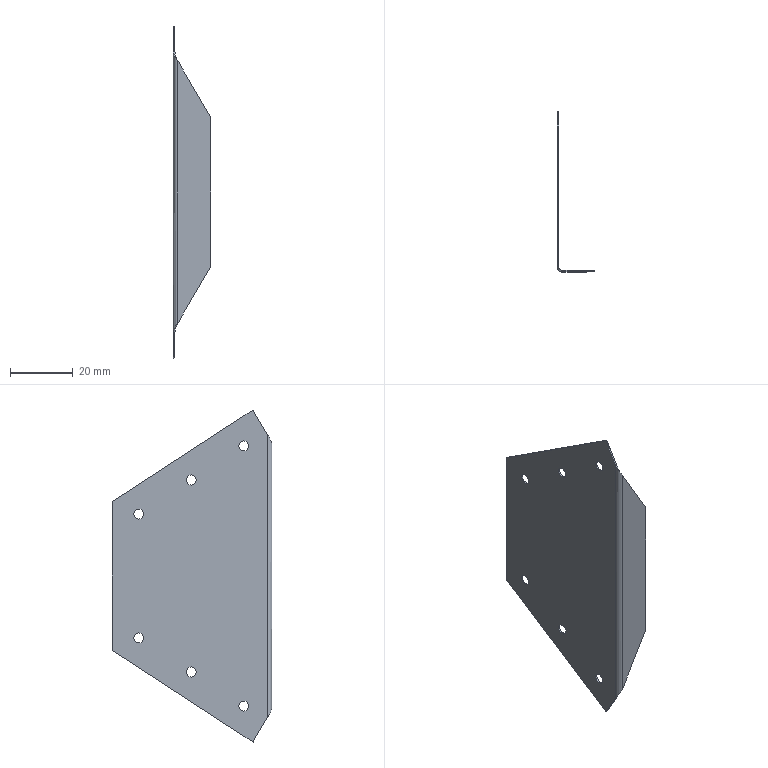Part | SolidWorks | features BaseBody 1 | 1 solid | 28 faces | box 12.018 x 51.018 x 106 mm | volume 2356 mm3 | cylinder 14 | plane 12 | spline 2 | commonest cylinder face diameters 3.2 x12 2 x1 3 x1
STEP:
#1=CARTESIAN_POINT('',(0.,-11.047,43.144));
#2=VERTEX_POINT('',#1);
#3=CARTESIAN_POINT('',(0.,-11.047,39.944));
#4=VERTEX_POINT('',#3);
#5=CARTESIAN_POINT('',(0.,-11.047,41.544));
#6=DIRECTION('',(1.,0.,0.));
#7=DIRECTION('',(0.,0.,1.));
#8=AXIS2_PLACEMENT_3D('',#5,#6,#7);
#9=CIRCLE('',#8,1.6);
#10=EDGE_CURVE('',#2,#4,#9,.T.);
#11=ORIENTED_EDGE('',*,*,#10,.T.);
#12=CARTESIAN_POINT('',(-0.5,-11.047,39.944));
#13=VERTEX_POINT('',#12);
#14=CARTESIAN_POINT('',(0.,-11.047,39.944));
#15=DIRECTION('',(-1.,0.,0.));
#16=VECTOR('',#15,1000.);
#17=LINE('',#14,#16);
#18=EDGE_CURVE('',#4,#13,#17,.T.);
#19=ORIENTED_EDGE('',*,*,#18,.T.);
#20=CARTESIAN_POINT('',(-0.5,-11.047,43.144));
#21=VERTEX_POINT('',#20);
#22=CARTESIAN_POINT('',(-0.5,-11.047,41.544));
#23=DIRECTION('',(-1.,0.,0.));
#24=DIRECTION('',(0.,0.,1.));
#25=AXIS2_PLACEMENT_3D('',#22,#23,#24);
#26=CIRCLE('',#25,1.6);
#27=EDGE_CURVE('',#13,#21,#26,.T.);
#28=ORIENTED_EDGE('',*,*,#27,.T.);
#29=CARTESIAN_POINT('',(0.,-11.047,43.144));
#30=DIRECTION('',(-1.,0.,0.));
#31=VECTOR('',#30,1000.);
#32=LINE('',#29,#31);
#33=EDGE_CURVE('',#2,#21,#32,.T.);
#34=ORIENTED_EDGE('',*,*,#33,.F.);
#35=EDGE_LOOP('',(#11,#19,#28,#34));
#36=FACE_OUTER_BOUND('',#35,.T.);
#37=CARTESIAN_POINT('',(0.,-11.047,41.544));
#38=DIRECTION('',(-1.,0.,0.));
#39=DIRECTION('',(0.,0.,1.));
#40=AXIS2_PLACEMENT_3D('',#37,#38,#39);
#41=CYLINDRICAL_SURFACE('',#40,1.6);
#42=ADVANCED_FACE('',(#36),#41,.F.);
#43=CARTESIAN_POINT('',(0.,-11.047,-43.144));
#44=VERTEX_POINT('',#43);
#45=CARTESIAN_POINT('',(0.,-11.047,-39.944));
#46=VERTEX_POINT('',#45);
#47=CARTESIAN_POINT('',(0.,-11.047,-41.544));
#48=DIRECTION('',(-1.,0.,0.));
#49=DIRECTION('',(0.,0.,1.));
#50=AXIS2_PLACEMENT_3D('',#47,#48,#49);
#51=CIRCLE('',#50,1.6);
#52=EDGE_CURVE('',#44,#46,#51,.T.);
#53=ORIENTED_EDGE('',*,*,#52,.F.);
#54=CARTESIAN_POINT('',(-0.5,-11.047,-43.144));
#55=VERTEX_POINT('',#54);
#56=CARTESIAN_POINT('',(0.,-11.047,-43.144));
#57=DIRECTION('',(-1.,0.,0.));
#58=VECTOR('',#57,1000.);
#59=LINE('',#56,#58);
#60=EDGE_CURVE('',#44,#55,#59,.T.);
#61=ORIENTED_EDGE('',*,*,#60,.T.);
#62=CARTESIAN_POINT('',(-0.5,-11.047,-39.944));
#63=VERTEX_POINT('',#62);
#64=CARTESIAN_POINT('',(-0.5,-11.047,-41.544));
#65=DIRECTION('',(-1.,0.,0.));
#66=DIRECTION('',(0.,0.,1.));
#67=AXIS2_PLACEMENT_3D('',#64,#65,#66);
#68=CIRCLE('',#67,1.6);
#69=EDGE_CURVE('',#55,#63,#68,.T.);
#70=ORIENTED_EDGE('',*,*,#69,.T.);
#71=CARTESIAN_POINT('',(0.,-11.047,-39.944));
#72=DIRECTION('',(-1.,0.,0.));
#73=VECTOR('',#72,1000.);
#74=LINE('',#71,#73);
#75=EDGE_CURVE('',#46,#63,#74,.T.);
#76=ORIENTED_EDGE('',*,*,#75,.F.);
#77=EDGE_LOOP('',(#53,#61,#70,#76));
#78=FACE_OUTER_BOUND('',#77,.T.);
#79=CARTESIAN_POINT('',(0.,-11.047,-41.544));
#80=DIRECTION('',(-1.,0.,0.));
#81=DIRECTION('',(0.,0.,1.));
#82=AXIS2_PLACEMENT_3D('',#79,#80,#81);
#83=CYLINDRICAL_SURFACE('',#82,1.6);
#84=ADVANCED_FACE('',(#78),#83,.F.);
#85=CARTESIAN_POINT('',(0.,5.726,-32.251));
#86=VERTEX_POINT('',#85);
#87=CARTESIAN_POINT('',(0.,5.726,-29.051));
#88=VERTEX_POINT('',#87);
#89=CARTESIAN_POINT('',(0.,5.726,-30.651));
#90=DIRECTION('',(-1.,0.,0.));
#91=DIRECTION('',(0.,0.,1.));
#92=AXIS2_PLACEMENT_3D('',#89,#90,#91);
#93=CIRCLE('',#92,1.6);
#94=EDGE_CURVE('',#86,#88,#93,.T.);
#95=ORIENTED_EDGE('',*,*,#94,.F.);
#96=CARTESIAN_POINT('',(-0.5,5.726,-32.251));
#97=VERTEX_POINT('',#96);
#98=CARTESIAN_POINT('',(0.,5.726,-32.251));
#99=DIRECTION('',(-1.,0.,0.));
#100=VECTOR('',#99,1000.);
#101=LINE('',#98,#100);
#102=EDGE_CURVE('',#86,#97,#101,.T.);
#103=ORIENTED_EDGE('',*,*,#102,.T.);
#104=CARTESIAN_POINT('',(-0.5,5.726,-29.051));
#105=VERTEX_POINT('',#104);
#106=CARTESIAN_POINT('',(-0.5,5.726,-30.651));
#107=DIRECTION('',(-1.,0.,0.));
#108=DIRECTION('',(0.,0.,1.));
#109=AXIS2_PLACEMENT_3D('',#106,#107,#108);
#110=CIRCLE('',#109,1.6);
#111=EDGE_CURVE('',#97,#105,#110,.T.);
#112=ORIENTED_EDGE('',*,*,#111,.T.);
#113=CARTESIAN_POINT('',(0.,5.726,-29.051));
#114=DIRECTION('',(-1.,0.,0.));
#115=VECTOR('',#114,1000.);
#116=LINE('',#113,#115);
#117=EDGE_CURVE('',#88,#105,#116,.T.);
#118=ORIENTED_EDGE('',*,*,#117,.F.);
#119=EDGE_LOOP('',(#95,#103,#112,#118));
#120=FACE_OUTER_BOUND('',#119,.T.);
#121=CARTESIAN_POINT('',(0.,5.726,-30.651));
#122=DIRECTION('',(-1.,0.,0.));
#123=DIRECTION('',(0.,0.,1.));
#124=AXIS2_PLACEMENT_3D('',#121,#122,#123);
#125=CYLINDRICAL_SURFACE('',#124,1.6);
#126=ADVANCED_FACE('',(#120),#125,.F.);
#127=CARTESIAN_POINT('',(0.,22.499,-21.358));
#128=VERTEX_POINT('',#127);
#129=CARTESIAN_POINT('',(0.,22.499,-18.158));
#130=VERTEX_POINT('',#129);
#131=CARTESIAN_POINT('',(0.,22.499,-19.758));
#132=DIRECTION('',(-1.,0.,0.));
#133=DIRECTION('',(0.,0.,1.));
#134=AXIS2_PLACEMENT_3D('',#131,#132,#133);
#135=CIRCLE('',#134,1.6);
#136=EDGE_CURVE('',#128,#130,#135,.T.);
#137=ORIENTED_EDGE('',*,*,#136,.F.);
#138=CARTESIAN_POINT('',(-0.5,22.499,-21.358));
#139=VERTEX_POINT('',#138);
#140=CARTESIAN_POINT('',(0.,22.499,-21.358));
#141=DIRECTION('',(-1.,0.,0.));
#142=VECTOR('',#141,1000.);
#143=LINE('',#140,#142);
#144=EDGE_CURVE('',#128,#139,#143,.T.);
#145=ORIENTED_EDGE('',*,*,#144,.T.);
#146=CARTESIAN_POINT('',(-0.5,22.499,-18.158));
#147=VERTEX_POINT('',#146);
#148=CARTESIAN_POINT('',(-0.5,22.499,-19.758));
#149=DIRECTION('',(-1.,0.,0.));
#150=DIRECTION('',(0.,0.,1.));
#151=AXIS2_PLACEMENT_3D('',#148,#149,#150);
#152=CIRCLE('',#151,1.6);
#153=EDGE_CURVE('',#139,#147,#152,.T.);
#154=ORIENTED_EDGE('',*,*,#153,.T.);
#155=CARTESIAN_POINT('',(0.,22.499,-18.158));
#156=DIRECTION('',(-1.,0.,0.));
#157=VECTOR('',#156,1000.);
#158=LINE('',#155,#157);
#159=EDGE_CURVE('',#130,#147,#158,.T.);
#160=ORIENTED_EDGE('',*,*,#159,.F.);
#161=EDGE_LOOP('',(#137,#145,#154,#160));
#162=FACE_OUTER_BOUND('',#161,.T.);
#163=CARTESIAN_POINT('',(0.,22.499,-19.758));
#164=DIRECTION('',(-1.,0.,0.));
#165=DIRECTION('',(0.,0.,1.));
#166=AXIS2_PLACEMENT_3D('',#163,#164,#165);
#167=CYLINDRICAL_SURFACE('',#166,1.6);
#168=ADVANCED_FACE('',(#162),#167,.F.);
#169=CARTESIAN_POINT('',(0.,22.499,18.158));
#170=VERTEX_POINT('',#169);
#171=CARTESIAN_POINT('',(0.,22.499,21.358));
#172=VERTEX_POINT('',#171);
#173=CARTESIAN_POINT('',(0.,22.499,19.758));
#174=DIRECTION('',(-1.,0.,0.));
#175=DIRECTION('',(0.,0.,1.));
#176=AXIS2_PLACEMENT_3D('',#173,#174,#175);
#177=CIRCLE('',#176,1.6);
#178=EDGE_CURVE('',#170,#172,#177,.T.);
#179=ORIENTED_EDGE('',*,*,#178,.F.);
#180=CARTESIAN_POINT('',(-0.5,22.499,18.158));
#181=VERTEX_POINT('',#180);
#182=CARTESIAN_POINT('',(0.,22.499,18.158));
#183=DIRECTION('',(-1.,0.,0.));
#184=VECTOR('',#183,1000.);
#185=LINE('',#182,#184);
#186=EDGE_CURVE('',#170,#181,#185,.T.);
#187=ORIENTED_EDGE('',*,*,#186,.T.);
#188=CARTESIAN_POINT('',(-0.5,22.499,21.358));
#189=VERTEX_POINT('',#188);
#190=CARTESIAN_POINT('',(-0.5,22.499,19.758));
#191=DIRECTION('',(-1.,0.,0.));
#192=DIRECTION('',(0.,0.,1.));
#193=AXIS2_PLACEMENT_3D('',#190,#191,#192);
#194=CIRCLE('',#193,1.6);
#195=EDGE_CURVE('',#181,#189,#194,.T.);
#196=ORIENTED_EDGE('',*,*,#195,.T.);
#197=CARTESIAN_POINT('',(0.,22.499,21.358));
#198=DIRECTION('',(-1.,0.,0.));
#199=VECTOR('',#198,1000.);
#200=LINE('',#197,#199);
#201=EDGE_CURVE('',#172,#189,#200,.T.);
#202=ORIENTED_EDGE('',*,*,#201,.F.);
#203=EDGE_LOOP('',(#179,#187,#196,#202));
#204=FACE_OUTER_BOUND('',#203,.T.);
#205=CARTESIAN_POINT('',(0.,22.499,19.758));
#206=DIRECTION('',(-1.,0.,0.));
#207=DIRECTION('',(0.,0.,1.));
#208=AXIS2_PLACEMENT_3D('',#205,#206,#207);
#209=CYLINDRICAL_SURFACE('',#208,1.6);
#210=ADVANCED_FACE('',(#204),#209,.F.);
#211=CARTESIAN_POINT('',(0.,5.726,29.051));
#212=VERTEX_POINT('',#211);
#213=CARTESIAN_POINT('',(0.,5.726,32.251));
#214=VERTEX_POINT('',#213);
#215=CARTESIAN_POINT('',(0.,5.726,30.651));
#216=DIRECTION('',(-1.,0.,0.));
#217=DIRECTION('',(0.,0.,1.));
#218=AXIS2_PLACEMENT_3D('',#215,#216,#217);
#219=CIRCLE('',#218,1.6);
#220=EDGE_CURVE('',#212,#214,#219,.T.);
#221=ORIENTED_EDGE('',*,*,#220,.F.);
#222=CARTESIAN_POINT('',(-0.5,5.726,29.051));
#223=VERTEX_POINT('',#222);
#224=CARTESIAN_POINT('',(0.,5.726,29.051));
#225=DIRECTION('',(-1.,0.,0.));
#226=VECTOR('',#225,1000.);
#227=LINE('',#224,#226);
#228=EDGE_CURVE('',#212,#223,#227,.T.);
#229=ORIENTED_EDGE('',*,*,#228,.T.);
#230=CARTESIAN_POINT('',(-0.5,5.726,32.251));
#231=VERTEX_POINT('',#230);
#232=CARTESIAN_POINT('',(-0.5,5.726,30.651));
#233=DIRECTION('',(-1.,0.,0.));
#234=DIRECTION('',(0.,0.,1.));
#235=AXIS2_PLACEMENT_3D('',#232,#233,#234);
#236=CIRCLE('',#235,1.6);
#237=EDGE_CURVE('',#223,#231,#236,.T.);
#238=ORIENTED_EDGE('',*,*,#237,.T.);
#239=CARTESIAN_POINT('',(0.,5.726,32.251));
#240=DIRECTION('',(-1.,0.,0.));
#241=VECTOR('',#240,1000.);
#242=LINE('',#239,#241);
#243=EDGE_CURVE('',#214,#231,#242,.T.);
#244=ORIENTED_EDGE('',*,*,#243,.F.);
#245=EDGE_LOOP('',(#221,#229,#238,#244));
#246=FACE_OUTER_BOUND('',#245,.T.);
#247=CARTESIAN_POINT('',(0.,5.726,30.651));
#248=DIRECTION('',(-1.,0.,0.));
#249=DIRECTION('',(0.,0.,1.));
#250=AXIS2_PLACEMENT_3D('',#247,#248,#249);
#251=CYLINDRICAL_SURFACE('',#250,1.6);
#252=ADVANCED_FACE('',(#246),#251,.F.);
#253=ORIENTED_EDGE('',*,*,#18,.F.);
#254=CARTESIAN_POINT('',(0.,-11.047,41.544));
#255=DIRECTION('',(1.,0.,0.));
#256=DIRECTION('',(0.,0.,1.));
#257=AXIS2_PLACEMENT_3D('',#254,#255,#256);
#258=CIRCLE('',#257,1.6);
#259=EDGE_CURVE('',#4,#2,#258,.T.);
#260=ORIENTED_EDGE('',*,*,#259,.T.);
#261=ORIENTED_EDGE('',*,*,#33,.T.);
#262=CARTESIAN_POINT('',(-0.5,-11.047,41.544));
#263=DIRECTION('',(-1.,0.,0.));
#264=DIRECTION('',(0.,0.,1.));
#265=AXIS2_PLACEMENT_3D('',#262,#263,#264);
#266=CIRCLE('',#265,1.6);
#267=EDGE_CURVE('',#21,#13,#266,.T.);
#268=ORIENTED_EDGE('',*,*,#267,.T.);
#269=EDGE_LOOP('',(#253,#260,#261,#268));
#270=FACE_OUTER_BOUND('',#269,.T.);
#271=CARTESIAN_POINT('',(0.,-11.047,41.544));
#272=DIRECTION('',(-1.,0.,0.));
#273=DIRECTION('',(0.,0.,1.));
#274=AXIS2_PLACEMENT_3D('',#271,#272,#273);
#275=CYLINDRICAL_SURFACE('',#274,1.6);
#276=ADVANCED_FACE('',(#270),#275,.F.);
#277=CARTESIAN_POINT('',(-0.5,-11.047,-41.544));
#278=DIRECTION('',(-1.,0.,0.));
#279=DIRECTION('',(0.,0.,1.));
#280=AXIS2_PLACEMENT_3D('',#277,#278,#279);
#281=CIRCLE('',#280,1.6);
#282=EDGE_CURVE('',#63,#55,#281,.T.);
#283=ORIENTED_EDGE('',*,*,#282,.F.);
#284=ORIENTED_EDGE('',*,*,#69,.F.);
#285=EDGE_LOOP('',(#283,#284));
#286=FACE_BOUND('',#285,.T.);
#287=CARTESIAN_POINT('',(-0.5,5.726,-30.651));
#288=DIRECTION('',(-1.,0.,0.));
#289=DIRECTION('',(0.,0.,1.));
#290=AXIS2_PLACEMENT_3D('',#287,#288,#289);
#291=CIRCLE('',#290,1.6);
#292=EDGE_CURVE('',#105,#97,#291,.T.);
#293=ORIENTED_EDGE('',*,*,#292,.F.);
#294=ORIENTED_EDGE('',*,*,#111,.F.);
#295=EDGE_LOOP('',(#293,#294));
#296=FACE_BOUND('',#295,.T.);
#297=CARTESIAN_POINT('',(-0.5,22.499,-19.758));
#298=DIRECTION('',(-1.,0.,0.));
#299=DIRECTION('',(0.,0.,1.));
#300=AXIS2_PLACEMENT_3D('',#297,#298,#299);
#301=CIRCLE('',#300,1.6);
#302=EDGE_CURVE('',#147,#139,#301,.T.);
#303=ORIENTED_EDGE('',*,*,#302,.F.);
#304=ORIENTED_EDGE('',*,*,#153,.F.);
#305=EDGE_LOOP('',(#303,#304));
#306=FACE_BOUND('',#305,.T.);
#307=CARTESIAN_POINT('',(-0.5,22.499,19.758));
#308=DIRECTION('',(-1.,0.,0.));
#309=DIRECTION('',(0.,0.,1.));
#310=AXIS2_PLACEMENT_3D('',#307,#308,#309);
#311=CIRCLE('',#310,1.6);
#312=EDGE_CURVE('',#189,#181,#311,.T.);
#313=ORIENTED_EDGE('',*,*,#312,.F.);
#314=ORIENTED_EDGE('',*,*,#195,.F.);
#315=EDGE_LOOP('',(#313,#314));
#316=FACE_BOUND('',#315,.T.);
#317=CARTESIAN_POINT('',(-0.5,5.726,30.651));
#318=DIRECTION('',(-1.,0.,0.));
#319=DIRECTION('',(0.,0.,1.));
#320=AXIS2_PLACEMENT_3D('',#317,#318,#319);
#321=CIRCLE('',#320,1.6);
#322=EDGE_CURVE('',#231,#223,#321,.T.);
#323=ORIENTED_EDGE('',*,*,#322,.F.);
#324=ORIENTED_EDGE('',*,*,#237,.F.);
#325=EDGE_LOOP('',(#323,#324));
#326=FACE_BOUND('',#325,.T.);
#327=ORIENTED_EDGE('',*,*,#267,.F.);
#328=ORIENTED_EDGE('',*,*,#27,.F.);
#329=EDGE_LOOP('',(#327,#328));
#330=FACE_BOUND('',#329,.T.);
#331=CARTESIAN_POINT('',(-0.5,-18.518,45.233));
#332=VERTEX_POINT('',#331);
#333=CARTESIAN_POINT('',(-0.5,-18.518,-45.233));
#334=VERTEX_POINT('',#333);
#335=CARTESIAN_POINT('',(-0.5,-18.518,0.));
#336=DIRECTION('',(0.,0.,-1.));
#337=VECTOR('',#336,1000.);
#338=LINE('',#335,#337);
#339=EDGE_CURVE('',#332,#334,#338,.T.);
#340=ORIENTED_EDGE('',*,*,#339,.F.);
#341=CARTESIAN_POINT('',(-0.5,-14.,53.));
#342=VERTEX_POINT('',#341);
#343=CARTESIAN_POINT('',(-0.5,-14.,53.));
#344=DIRECTION('',(0.,-0.5028,-0.8644));
#345=VECTOR('',#344,1000.);
#346=LINE('',#343,#345);
#347=EDGE_CURVE('',#342,#332,#346,.T.);
#348=ORIENTED_EDGE('',*,*,#347,.F.);
#349=CARTESIAN_POINT('',(-0.5,31.,23.777));
#350=VERTEX_POINT('',#349);
#351=CARTESIAN_POINT('',(-0.5,31.,23.777));
#352=DIRECTION('',(0.,-0.8387,0.5446));
#353=VECTOR('',#352,1000.);
#354=LINE('',#351,#353);
#355=EDGE_CURVE('',#350,#342,#354,.T.);
#356=ORIENTED_EDGE('',*,*,#355,.F.);
#357=CARTESIAN_POINT('',(-0.5,31.,-23.777));
#358=VERTEX_POINT('',#357);
#359=CARTESIAN_POINT('',(-0.5,31.,0.));
#360=DIRECTION('',(0.,0.,1.));
#361=VECTOR('',#360,1000.);
#362=LINE('',#359,#361);
#363=EDGE_CURVE('',#358,#350,#362,.T.);
#364=ORIENTED_EDGE('',*,*,#363,.F.);
#365=CARTESIAN_POINT('',(-0.5,-14.,-53.));
#366=VERTEX_POINT('',#365);
#367=CARTESIAN_POINT('',(-0.5,-14.,-53.));
#368=DIRECTION('',(0.,0.8387,0.5446));
#369=VECTOR('',#368,1000.);
#370=LINE('',#367,#369);
#371=EDGE_CURVE('',#366,#358,#370,.T.);
#372=ORIENTED_EDGE('',*,*,#371,.F.);
#373=CARTESIAN_POINT('',(-0.5,-18.518,-45.233));
#374=DIRECTION('',(0.,0.5028,-0.8644));
#375=VECTOR('',#374,1000.);
#376=LINE('',#373,#375);
#377=EDGE_CURVE('',#334,#366,#376,.T.);
#378=ORIENTED_EDGE('',*,*,#377,.F.);
#379=EDGE_LOOP('',(#340,#348,#356,#364,#372,#378));
#380=FACE_OUTER_BOUND('',#379,.T.);
#381=CARTESIAN_POINT('',(-0.5,-18.518,53.636));
#382=DIRECTION('',(1.,0.,0.));
#383=DIRECTION('',(0.,0.,-1.));
#384=AXIS2_PLACEMENT_3D('',#381,#382,#383);
#385=PLANE('',#384);
#386=ADVANCED_FACE('',(#286,#296,#306,#316,#326,#330,#380),#385,.F.);
#387=CARTESIAN_POINT('',(0.,-11.047,-41.544));
#388=DIRECTION('',(-1.,0.,0.));
#389=DIRECTION('',(0.,0.,1.));
#390=AXIS2_PLACEMENT_3D('',#387,#388,#389);
#391=CIRCLE('',#390,1.6);
#392=EDGE_CURVE('',#46,#44,#391,.T.);
#393=ORIENTED_EDGE('',*,*,#392,.T.);
#394=ORIENTED_EDGE('',*,*,#52,.T.);
#395=EDGE_LOOP('',(#393,#394));
#396=FACE_BOUND('',#395,.T.);
#397=CARTESIAN_POINT('',(0.,5.726,-30.651));
#398=DIRECTION('',(-1.,0.,0.));
#399=DIRECTION('',(0.,0.,1.));
#400=AXIS2_PLACEMENT_3D('',#397,#398,#399);
#401=CIRCLE('',#400,1.6);
#402=EDGE_CURVE('',#88,#86,#401,.T.);
#403=ORIENTED_EDGE('',*,*,#402,.T.);
#404=ORIENTED_EDGE('',*,*,#94,.T.);
#405=EDGE_LOOP('',(#403,#404));
#406=FACE_BOUND('',#405,.T.);
#407=CARTESIAN_POINT('',(0.,22.499,-19.758));
#408=DIRECTION('',(-1.,0.,0.));
#409=DIRECTION('',(0.,0.,1.));
#410=AXIS2_PLACEMENT_3D('',#407,#408,#409);
#411=CIRCLE('',#410,1.6);
#412=EDGE_CURVE('',#130,#128,#411,.T.);
#413=ORIENTED_EDGE('',*,*,#412,.T.);
#414=ORIENTED_EDGE('',*,*,#136,.T.);
#415=EDGE_LOOP('',(#413,#414));
#416=FACE_BOUND('',#415,.T.);
#417=CARTESIAN_POINT('',(0.,22.499,19.758));
#418=DIRECTION('',(-1.,0.,0.));
#419=DIRECTION('',(0.,0.,1.));
#420=AXIS2_PLACEMENT_3D('',#417,#418,#419);
#421=CIRCLE('',#420,1.6);
#422=EDGE_CURVE('',#172,#170,#421,.T.);
#423=ORIENTED_EDGE('',*,*,#422,.T.);
#424=ORIENTED_EDGE('',*,*,#178,.T.);
#425=EDGE_LOOP('',(#423,#424));
#426=FACE_BOUND('',#425,.T.);
#427=CARTESIAN_POINT('',(0.,5.726,30.651));
#428=DIRECTION('',(-1.,0.,0.));
#429=DIRECTION('',(0.,0.,1.));
#430=AXIS2_PLACEMENT_3D('',#427,#428,#429);
#431=CIRCLE('',#430,1.6);
#432=EDGE_CURVE('',#214,#212,#431,.T.);
#433=ORIENTED_EDGE('',*,*,#432,.T.);
#434=ORIENTED_EDGE('',*,*,#220,.T.);
#435=EDGE_LOOP('',(#433,#434));
#436=FACE_BOUND('',#435,.T.);
#437=ORIENTED_EDGE('',*,*,#10,.F.);
#438=ORIENTED_EDGE('',*,*,#259,.F.);
#439=EDGE_LOOP('',(#437,#438));
#440=FACE_BOUND('',#439,.T.);
#441=CARTESIAN_POINT('',(0.,31.,23.777));
#442=VERTEX_POINT('',#441);
#443=CARTESIAN_POINT('',(0.,-14.,53.));
#444=VERTEX_POINT('',#443);
#445=CARTESIAN_POINT('',(0.,31.,23.777));
#446=DIRECTION('',(0.,-0.8387,0.5446));
#447=VECTOR('',#446,1000.);
#448=LINE('',#445,#447);
#449=EDGE_CURVE('',#442,#444,#448,.T.);
#450=ORIENTED_EDGE('',*,*,#449,.T.);
#451=CARTESIAN_POINT('',(0.,-18.518,45.233));
#452=VERTEX_POINT('',#451);
#453=CARTESIAN_POINT('',(0.,-14.,53.));
#454=DIRECTION('',(0.,-0.5028,-0.8644));
#455=VECTOR('',#454,1000.);
#456=LINE('',#453,#455);
#457=EDGE_CURVE('',#444,#452,#456,.T.);
#458=ORIENTED_EDGE('',*,*,#457,.T.);
#459=CARTESIAN_POINT('',(0.,-18.518,-45.233));
#460=VERTEX_POINT('',#459);
#461=CARTESIAN_POINT('',(0.,-18.518,0.));
#462=DIRECTION('',(0.,0.,-1.));
#463=VECTOR('',#462,1000.);
#464=LINE('',#461,#463);
#465=EDGE_CURVE('',#452,#460,#464,.T.);
#466=ORIENTED_EDGE('',*,*,#465,.T.);
#467=CARTESIAN_POINT('',(0.,-14.,-53.));
#468=VERTEX_POINT('',#467);
#469=CARTESIAN_POINT('',(0.,-18.518,-45.233));
#470=DIRECTION('',(0.,0.5028,-0.8644));
#471=VECTOR('',#470,1000.);
#472=LINE('',#469,#471);
#473=EDGE_CURVE('',#460,#468,#472,.T.);
#474=ORIENTED_EDGE('',*,*,#473,.T.);
#475=CARTESIAN_POINT('',(0.,31.,-23.777));
#476=VERTEX_POINT('',#475);
#477=CARTESIAN_POINT('',(0.,-14.,-53.));
#478=DIRECTION('',(0.,0.8387,0.5446));
#479=VECTOR('',#478,1000.);
#480=LINE('',#477,#479);
#481=EDGE_CURVE('',#468,#476,#480,.T.);
#482=ORIENTED_EDGE('',*,*,#481,.T.);
#483=CARTESIAN_POINT('',(0.,31.,0.));
#484=DIRECTION('',(0.,0.,1.));
#485=VECTOR('',#484,1000.);
#486=LINE('',#483,#485);
#487=EDGE_CURVE('',#476,#442,#486,.T.);
#488=ORIENTED_EDGE('',*,*,#487,.T.);
#489=EDGE_LOOP('',(#450,#458,#466,#474,#482,#488));
#490=FACE_OUTER_BOUND('',#489,.T.);
#491=CARTESIAN_POINT('',(0.,-18.518,53.636));
#492=DIRECTION('',(1.,0.,0.));
#493=DIRECTION('',(0.,0.,-1.));
#494=AXIS2_PLACEMENT_3D('',#491,#492,#493);
#495=PLANE('',#494);
#496=ADVANCED_FACE('',(#396,#406,#416,#426,#436,#440,#490),#495,.T.);
#497=ORIENTED_EDGE('',*,*,#60,.F.);
#498=ORIENTED_EDGE('',*,*,#392,.F.);
#499=ORIENTED_EDGE('',*,*,#75,.T.);
#500=ORIENTED_EDGE('',*,*,#282,.T.);
#501=EDGE_LOOP('',(#497,#498,#499,#500));
#502=FACE_OUTER_BOUND('',#501,.T.);
#503=CARTESIAN_POINT('',(0.,-11.047,-41.544));
#504=DIRECTION('',(-1.,0.,0.));
#505=DIRECTION('',(0.,0.,1.));
#506=AXIS2_PLACEMENT_3D('',#503,#504,#505);
#507=CYLINDRICAL_SURFACE('',#506,1.6);
#508=ADVANCED_FACE('',(#502),#507,.F.);
#509=ORIENTED_EDGE('',*,*,#102,.F.);
#510=ORIENTED_EDGE('',*,*,#402,.F.);
#511=ORIENTED_EDGE('',*,*,#117,.T.);
#512=ORIENTED_EDGE('',*,*,#292,.T.);
#513=EDGE_LOOP('',(#509,#510,#511,#512));
#514=FACE_OUTER_BOUND('',#513,.T.);
#515=CARTESIAN_POINT('',(0.,5.726,-30.651));
#516=DIRECTION('',(-1.,0.,0.));
#517=DIRECTION('',(0.,0.,1.));
#518=AXIS2_PLACEMENT_3D('',#515,#516,#517);
#519=CYLINDRICAL_SURFACE('',#518,1.6);
#520=ADVANCED_FACE('',(#514),#519,.F.);
#521=ORIENTED_EDGE('',*,*,#144,.F.);
#522=ORIENTED_EDGE('',*,*,#412,.F.);
#523=ORIENTED_EDGE('',*,*,#159,.T.);
#524=ORIENTED_EDGE('',*,*,#302,.T.);
#525=EDGE_LOOP('',(#521,#522,#523,#524));
#526=FACE_OUTER_BOUND('',#525,.T.);
#527=CARTESIAN_POINT('',(0.,22.499,-19.758));
#528=DIRECTION('',(-1.,0.,0.));
#529=DIRECTION('',(0.,0.,1.));
#530=AXIS2_PLACEMENT_3D('',#527,#528,#529);
#531=CYLINDRICAL_SURFACE('',#530,1.6);
#532=ADVANCED_FACE('',(#526),#531,.F.);
#533=ORIENTED_EDGE('',*,*,#186,.F.);
#534=ORIENTED_EDGE('',*,*,#422,.F.);
#535=ORIENTED_EDGE('',*,*,#201,.T.);
#536=ORIENTED_EDGE('',*,*,#312,.T.);
#537=EDGE_LOOP('',(#533,#534,#535,#536));
#538=FACE_OUTER_BOUND('',#537,.T.);
#539=CARTESIAN_POINT('',(0.,22.499,19.758));
#540=DIRECTION('',(-1.,0.,0.));
#541=DIRECTION('',(0.,0.,1.));
#542=AXIS2_PLACEMENT_3D('',#539,#540,#541);
#543=CYLINDRICAL_SURFACE('',#542,1.6);
#544=ADVANCED_FACE('',(#538),#543,.F.);
#545=ORIENTED_EDGE('',*,*,#228,.F.);
#546=ORIENTED_EDGE('',*,*,#432,.F.);
#547=ORIENTED_EDGE('',*,*,#243,.T.);
#548=ORIENTED_EDGE('',*,*,#322,.T.);
#549=EDGE_LOOP('',(#545,#546,#547,#548));
#550=FACE_OUTER_BOUND('',#549,.T.);
#551=CARTESIAN_POINT('',(0.,5.726,30.651));
#552=DIRECTION('',(-1.,0.,0.));
#553=DIRECTION('',(0.,0.,1.));
#554=AXIS2_PLACEMENT_3D('',#551,#552,#553);
#555=CYLINDRICAL_SURFACE('',#554,1.6);
#556=ADVANCED_FACE('',(#550),#555,.F.);
#557=CARTESIAN_POINT('',(-0.25,-14.,-53.));
#558=DIRECTION('',(1.,0.,0.));
#559=VECTOR('',#558,1000.);
#560=LINE('',#557,#559);
#561=EDGE_CURVE('',#366,#468,#560,.T.);
#562=ORIENTED_EDGE('',*,*,#561,.T.);
#563=ORIENTED_EDGE('',*,*,#473,.F.);
#564=CARTESIAN_POINT('',(-0.25,-18.518,-45.233));
#565=DIRECTION('',(1.,0.,0.));
#566=VECTOR('',#565,1000.);
#567=LINE('',#564,#566);
#568=EDGE_CURVE('',#334,#460,#567,.T.);
#569=ORIENTED_EDGE('',*,*,#568,.F.);
#570=ORIENTED_EDGE('',*,*,#377,.T.);
#571=EDGE_LOOP('',(#562,#563,#569,#570));
#572=FACE_OUTER_BOUND('',#571,.T.);
#573=CARTESIAN_POINT('',(-0.5,-18.518,-45.233));
#574=DIRECTION('',(0.,-0.8644,-0.5028));
#575=DIRECTION('',(0.,0.5028,-0.8644));
#576=AXIS2_PLACEMENT_3D('',#573,#574,#575);
#577=PLANE('',#576);
#578=ADVANCED_FACE('',(#572),#577,.T.);
#579=ORIENTED_EDGE('',*,*,#339,.T.);
#580=CARTESIAN_POINT('',(1.,-20.018,-41.858));
#581=VERTEX_POINT('',#580);
#582=CARTESIAN_POINT('',(1.,-20.018,-41.858));
#583=CARTESIAN_POINT('',(0.802,-20.018,-42.141));
#584=CARTESIAN_POINT('',(0.6064,-19.979,-42.422));
#585=CARTESIAN_POINT('',(0.2411,-19.827,-42.988));
#586=CARTESIAN_POINT('',(0.07684,-19.717,-43.267));
#587=CARTESIAN_POINT('',(-0.1995,-19.44,-43.827));
#588=CARTESIAN_POINT('',(-0.3117,-19.272,-44.111));
#589=CARTESIAN_POINT('',(-0.461,-18.91,-44.671));
#590=CARTESIAN_POINT('',(-0.5,-18.716,-44.949));
#591=CARTESIAN_POINT('',(-0.5,-18.518,-45.233));
#592=B_SPLINE_CURVE_WITH_KNOTS('',3,(#582,#583,#584,#585,#586,#587,#588,#589,#590,#591),.UNSPECIFIED.,.F.,.F.,(4,2,2,2,4),(0.,0.001031,0.002062,0.003093,0.004125),.UNSPECIFIED.);
#593=EDGE_CURVE('',#581,#334,#592,.T.);
#594=ORIENTED_EDGE('',*,*,#593,.F.);
#595=CARTESIAN_POINT('',(1.,-20.018,41.858));
#596=VERTEX_POINT('',#595);
#597=CARTESIAN_POINT('',(1.,-20.018,0.));
#598=DIRECTION('',(0.,0.,-1.));
#599=VECTOR('',#598,1000.);
#600=LINE('',#597,#599);
#601=EDGE_CURVE('',#596,#581,#600,.T.);
#602=ORIENTED_EDGE('',*,*,#601,.F.);
#603=CARTESIAN_POINT('',(-0.5,-18.518,45.233));
#604=CARTESIAN_POINT('',(-0.5,-18.721,44.953));
#605=CARTESIAN_POINT('',(-0.4593,-18.915,44.671));
#606=CARTESIAN_POINT('',(-0.3113,-19.272,44.098));
#607=CARTESIAN_POINT('',(-0.2065,-19.428,43.813));
#608=CARTESIAN_POINT('',(0.0499,-19.694,43.239));
#609=CARTESIAN_POINT('',(0.2103,-19.809,42.951));
#610=CARTESIAN_POINT('',(0.5754,-19.971,42.395));
#611=CARTESIAN_POINT('',(0.7797,-20.018,42.126));
#612=CARTESIAN_POINT('',(1.,-20.018,41.858));
#613=B_SPLINE_CURVE_WITH_KNOTS('',3,(#603,#604,#605,#606,#607,#608,#609,#610,#611,#612),.UNSPECIFIED.,.F.,.F.,(4,2,2,2,4),(0.,0.001032,0.002063,0.003095,0.004126),.UNSPECIFIED.);
#614=EDGE_CURVE('',#332,#596,#613,.T.);
#615=ORIENTED_EDGE('',*,*,#614,.F.);
#616=EDGE_LOOP('',(#579,#594,#602,#615));
#617=FACE_OUTER_BOUND('',#616,.T.);
#618=CARTESIAN_POINT('',(1.,-18.518,-45.776));
#619=DIRECTION('',(0.,0.,1.));
#620=DIRECTION('',(1.,0.,0.));
#621=AXIS2_PLACEMENT_3D('',#618,#619,#620);
#622=CYLINDRICAL_SURFACE('',#621,1.5);
#623=ADVANCED_FACE('',(#617),#622,.T.);
#624=CARTESIAN_POINT('',(-0.25,-14.,53.));
#625=DIRECTION('',(-1.,0.,0.));
#626=VECTOR('',#625,1000.);
#627=LINE('',#624,#626);
#628=EDGE_CURVE('',#444,#342,#627,.T.);
#629=ORIENTED_EDGE('',*,*,#628,.T.);
#630=ORIENTED_EDGE('',*,*,#347,.T.);
#631=CARTESIAN_POINT('',(-0.25,-18.518,45.233));
#632=DIRECTION('',(1.,0.,0.));
#633=VECTOR('',#632,1000.);
#634=LINE('',#631,#633);
#635=EDGE_CURVE('',#332,#452,#634,.T.);
#636=ORIENTED_EDGE('',*,*,#635,.T.);
#637=ORIENTED_EDGE('',*,*,#457,.F.);
#638=EDGE_LOOP('',(#629,#630,#636,#637));
#639=FACE_OUTER_BOUND('',#638,.T.);
#640=CARTESIAN_POINT('',(-0.5,-14.,53.));
#641=DIRECTION('',(0.,-0.8644,0.5028));
#642=DIRECTION('',(0.,-0.5028,-0.8644));
#643=AXIS2_PLACEMENT_3D('',#640,#641,#642);
#644=PLANE('',#643);
#645=ADVANCED_FACE('',(#639),#644,.T.);
#646=ORIENTED_EDGE('',*,*,#355,.T.);
#647=ORIENTED_EDGE('',*,*,#628,.F.);
#648=ORIENTED_EDGE('',*,*,#449,.F.);
#649=CARTESIAN_POINT('',(-0.25,31.,23.777));
#650=DIRECTION('',(-1.,0.,0.));
#651=VECTOR('',#650,1000.);
#652=LINE('',#649,#651);
#653=EDGE_CURVE('',#442,#350,#652,.T.);
#654=ORIENTED_EDGE('',*,*,#653,.T.);
#655=EDGE_LOOP('',(#646,#647,#648,#654));
#656=FACE_OUTER_BOUND('',#655,.T.);
#657=CARTESIAN_POINT('',(-0.5,31.,23.777));
#658=DIRECTION('',(0.,0.5446,0.8387));
#659=DIRECTION('',(0.,-0.8387,0.5446));
#660=AXIS2_PLACEMENT_3D('',#657,#658,#659);
#661=PLANE('',#660);
#662=ADVANCED_FACE('',(#656),#661,.T.);
#663=ORIENTED_EDGE('',*,*,#363,.T.);
#664=ORIENTED_EDGE('',*,*,#653,.F.);
#665=ORIENTED_EDGE('',*,*,#487,.F.);
#666=CARTESIAN_POINT('',(-0.25,31.,-23.777));
#667=DIRECTION('',(-1.,0.,0.));
#668=VECTOR('',#667,1000.);
#669=LINE('',#666,#668);
#670=EDGE_CURVE('',#476,#358,#669,.T.);
#671=ORIENTED_EDGE('',*,*,#670,.T.);
#672=EDGE_LOOP('',(#663,#664,#665,#671));
#673=FACE_OUTER_BOUND('',#672,.T.);
#674=CARTESIAN_POINT('',(-0.5,31.,-23.777));
#675=DIRECTION('',(0.,1.,0.));
#676=DIRECTION('',(0.,0.,1.));
#677=AXIS2_PLACEMENT_3D('',#674,#675,#676);
#678=PLANE('',#677);
#679=ADVANCED_FACE('',(#673),#678,.T.);
#680=ORIENTED_EDGE('',*,*,#371,.T.);
#681=ORIENTED_EDGE('',*,*,#670,.F.);
#682=ORIENTED_EDGE('',*,*,#481,.F.);
#683=ORIENTED_EDGE('',*,*,#561,.F.);
#684=EDGE_LOOP('',(#680,#681,#682,#683));
#685=FACE_OUTER_BOUND('',#684,.T.);
#686=CARTESIAN_POINT('',(-0.5,-14.,-53.));
#687=DIRECTION('',(0.,0.5446,-0.8387));
#688=DIRECTION('',(0.,0.8387,0.5446));
#689=AXIS2_PLACEMENT_3D('',#686,#687,#688);
#690=PLANE('',#689);
#691=ADVANCED_FACE('',(#685),#690,.T.);
#692=CARTESIAN_POINT('',(1.,-19.518,-41.858));
#693=VERTEX_POINT('',#692);
#694=CARTESIAN_POINT('',(1.,-19.518,-41.858));
#695=CARTESIAN_POINT('',(0.8684,-19.518,-42.14));
#696=CARTESIAN_POINT('',(0.7379,-19.492,-42.421));
#697=CARTESIAN_POINT('',(0.4952,-19.391,-42.986));
#698=CARTESIAN_POINT('',(0.3842,-19.317,-43.267));
#699=CARTESIAN_POINT('',(0.1988,-19.131,-43.832));
#700=CARTESIAN_POINT('',(0.1253,-19.02,-44.112));
#701=CARTESIAN_POINT('',(0.02605,-18.78,-44.671));
#702=CARTESIAN_POINT('',(0.000000001,-18.65,-44.95));
#703=CARTESIAN_POINT('',(0.,-18.518,-45.233));
#704=B_SPLINE_CURVE_WITH_KNOTS('',3,(#694,#695,#696,#697,#698,#699,#700,#701,#702,#703),.UNSPECIFIED.,.F.,.F.,(4,2,2,2,4),(0.,0.0009316,0.001863,0.002795,0.003727),.UNSPECIFIED.);
#705=EDGE_CURVE('',#693,#460,#704,.T.);
#706=ORIENTED_EDGE('',*,*,#705,.T.);
#707=ORIENTED_EDGE('',*,*,#465,.F.);
#708=CARTESIAN_POINT('',(1.,-19.518,41.858));
#709=VERTEX_POINT('',#708);
#710=CARTESIAN_POINT('',(0.,-18.518,45.233));
#711=CARTESIAN_POINT('',(0.000000001,-18.789,44.671));
#712=CARTESIAN_POINT('',(0.1096,-19.035,44.104));
#713=CARTESIAN_POINT('',(0.3643,-19.3,43.246));
#714=CARTESIAN_POINT('',(0.4692,-19.376,42.962));
#715=CARTESIAN_POINT('',(0.7116,-19.485,42.406));
#716=CARTESIAN_POINT('',(0.8496,-19.518,42.132));
#717=CARTESIAN_POINT('',(1.,-19.518,41.858));
#718=B_SPLINE_CURVE_WITH_KNOTS('',3,(#710,#711,#712,#713,#714,#715,#716,#717),.UNSPECIFIED.,.F.,.F.,(4,2,2,4),(0.,0.001863,0.002795,0.003727),.UNSPECIFIED.);
#719=EDGE_CURVE('',#452,#709,#718,.T.);
#720=ORIENTED_EDGE('',*,*,#719,.T.);
#721=CARTESIAN_POINT('',(1.,-19.518,0.));
#722=DIRECTION('',(0.,0.,-1.));
#723=VECTOR('',#722,1000.);
#724=LINE('',#721,#723);
#725=EDGE_CURVE('',#709,#693,#724,.T.);
#726=ORIENTED_EDGE('',*,*,#725,.T.);
#727=EDGE_LOOP('',(#706,#707,#720,#726));
#728=FACE_OUTER_BOUND('',#727,.T.);
#729=CARTESIAN_POINT('',(1.,-18.518,-45.776));
#730=DIRECTION('',(0.,0.,1.));
#731=DIRECTION('',(1.,0.,0.));
#732=AXIS2_PLACEMENT_3D('',#729,#730,#731);
#733=CYLINDRICAL_SURFACE('',#732,1.);
#734=ADVANCED_FACE('',(#728),#733,.F.);
#735=ORIENTED_EDGE('',*,*,#635,.F.);
#736=ORIENTED_EDGE('',*,*,#614,.T.);
#737=CARTESIAN_POINT('',(1.,-19.768,41.858));
#738=DIRECTION('',(0.,-1.,0.));
#739=VECTOR('',#738,1000.);
#740=LINE('',#737,#739);
#741=EDGE_CURVE('',#709,#596,#740,.T.);
#742=ORIENTED_EDGE('',*,*,#741,.F.);
#743=ORIENTED_EDGE('',*,*,#719,.F.);
#744=EDGE_LOOP('',(#735,#736,#742,#743));
#745=FACE_OUTER_BOUND('',#744,.T.);
#746=CARTESIAN_POINT('',(1.,-20.023,41.858));
#747=CARTESIAN_POINT('',(0.7957,-20.023,42.105));
#748=CARTESIAN_POINT('',(0.5915,-19.981,42.371));
#749=CARTESIAN_POINT('',(0.3102,-19.86,42.795));
#750=CARTESIAN_POINT('',(0.2205,-19.81,42.94));
#751=CARTESIAN_POINT('',(0.09504,-19.722,43.166));
#752=CARTESIAN_POINT('',(0.0547,-19.69,43.242));
#753=CARTESIAN_POINT('',(-0.02259,-19.624,43.396));
#754=CARTESIAN_POINT('',(-0.05923,-19.589,43.474));
#755=CARTESIAN_POINT('',(-0.236,-19.401,43.875));
#756=CARTESIAN_POINT('',(-0.3403,-19.229,44.175));
#757=CARTESIAN_POINT('',(-0.4747,-18.874,44.735));
#758=CARTESIAN_POINT('',(-0.505,-18.692,44.994));
#759=CARTESIAN_POINT('',(-0.505,-18.518,45.233));
#760=CARTESIAN_POINT('',(1.,-20.018,41.858));
#761=CARTESIAN_POINT('',(0.7964,-20.018,42.105));
#762=CARTESIAN_POINT('',(0.5929,-19.976,42.371));
#763=CARTESIAN_POINT('',(0.3125,-19.855,42.795));
#764=CARTESIAN_POINT('',(0.2231,-19.805,42.94));
#765=CARTESIAN_POINT('',(0.09805,-19.718,43.166));
#766=CARTESIAN_POINT('',(0.05784,-19.687,43.242));
#767=CARTESIAN_POINT('',(-0.01919,-19.62,43.396));
#768=CARTESIAN_POINT('',(-0.05571,-19.585,43.474));
#769=CARTESIAN_POINT('',(-0.2319,-19.398,43.875));
#770=CARTESIAN_POINT('',(-0.3358,-19.226,44.175));
#771=CARTESIAN_POINT('',(-0.4698,-18.873,44.735));
#772=CARTESIAN_POINT('',(-0.5,-18.691,44.994));
#773=CARTESIAN_POINT('',(-0.5,-18.518,45.233));
#774=CARTESIAN_POINT('',(1.,-19.518,41.858));
#775=CARTESIAN_POINT('',(0.8643,-19.518,42.105));
#776=CARTESIAN_POINT('',(0.7286,-19.49,42.371));
#777=CARTESIAN_POINT('',(0.5417,-19.41,42.795));
#778=CARTESIAN_POINT('',(0.4821,-19.376,42.94));
#779=CARTESIAN_POINT('',(0.3987,-19.318,43.166));
#780=CARTESIAN_POINT('',(0.3719,-19.297,43.242));
#781=CARTESIAN_POINT('',(0.3205,-19.253,43.396));
#782=CARTESIAN_POINT('',(0.2962,-19.229,43.474));
#783=CARTESIAN_POINT('',(0.1788,-19.105,43.875));
#784=CARTESIAN_POINT('',(0.1095,-18.99,44.175));
#785=CARTESIAN_POINT('',(0.02016,-18.755,44.735));
#786=CARTESIAN_POINT('',(0.,-18.633,44.994));
#787=CARTESIAN_POINT('',(0.,-18.518,45.233));
#788=CARTESIAN_POINT('',(1.,-19.513,41.858));
#789=CARTESIAN_POINT('',(0.865,-19.513,42.105));
#790=CARTESIAN_POINT('',(0.73,-19.485,42.371));
#791=CARTESIAN_POINT('',(0.544,-19.405,42.795));
#792=CARTESIAN_POINT('',(0.4847,-19.372,42.94));
#793=CARTESIAN_POINT('',(0.4017,-19.314,43.166));
#794=CARTESIAN_POINT('',(0.3751,-19.293,43.242));
#795=CARTESIAN_POINT('',(0.324,-19.249,43.396));
#796=CARTESIAN_POINT('',(0.2997,-19.226,43.474));
#797=CARTESIAN_POINT('',(0.1829,-19.102,43.875));
#798=CARTESIAN_POINT('',(0.114,-18.988,44.175));
#799=CARTESIAN_POINT('',(0.02511,-18.753,44.735));
#800=CARTESIAN_POINT('',(0.00505,-18.633,44.994));
#801=CARTESIAN_POINT('',(0.00505,-18.518,45.233));
#802=B_SPLINE_SURFACE_WITH_KNOTS('',1,3,((#746,#747,#748,#749,#750,#751,#752,#753,#754,#755,#756,#757,#758,#759),(#760,#761,#762,#763,#764,#765,#766,#767,#768,#769,#770,#771,#772,#773),(#774,#775,#776,#777,#778,#779,#780,#781,#782,#783,#784,#785,#786,#787),(#788,#789,#790,#791,#792,#793,#794,#795,#796,#797,#798,#799,#800,#801)),.UNSPECIFIED.,.F.,.F.,.F.,(2,1,1,2),(4,2,2,2,2,2,4),(-0.01,0.,1.,1.01),(0.,0.25,0.375,0.4375,0.5,0.75,1.),.UNSPECIFIED.);
#803=ADVANCED_FACE('',(#745),#802,.T.);
#804=CARTESIAN_POINT('',(1.,-19.768,-41.858));
#805=DIRECTION('',(0.,1.,0.));
#806=VECTOR('',#805,1000.);
#807=LINE('',#804,#806);
#808=EDGE_CURVE('',#581,#693,#807,.T.);
#809=ORIENTED_EDGE('',*,*,#808,.F.);
#810=ORIENTED_EDGE('',*,*,#593,.T.);
#811=ORIENTED_EDGE('',*,*,#568,.T.);
#812=ORIENTED_EDGE('',*,*,#705,.F.);
#813=EDGE_LOOP('',(#809,#810,#811,#812));
#814=FACE_OUTER_BOUND('',#813,.T.);
#815=CARTESIAN_POINT('',(-0.505,-18.518,-45.233));
#816=CARTESIAN_POINT('',(-0.505,-18.715,-44.952));
#817=CARTESIAN_POINT('',(-0.4658,-18.912,-44.67));
#818=CARTESIAN_POINT('',(-0.315,-19.276,-44.108));
#819=CARTESIAN_POINT('',(-0.2035,-19.443,-43.827));
#820=CARTESIAN_POINT('',(0.07511,-19.722,-43.264));
#821=CARTESIAN_POINT('',(0.2421,-19.833,-42.983));
#822=CARTESIAN_POINT('',(0.6061,-19.984,-42.42));
#823=CARTESIAN_POINT('',(0.803,-20.023,-42.139));
#824=CARTESIAN_POINT('',(1.,-20.023,-41.858));
#825=CARTESIAN_POINT('',(-0.5,-18.518,-45.233));
#826=CARTESIAN_POINT('',(-0.5,-18.715,-44.952));
#827=CARTESIAN_POINT('',(-0.461,-18.911,-44.67));
#828=CARTESIAN_POINT('',(-0.3107,-19.274,-44.108));
#829=CARTESIAN_POINT('',(-0.1995,-19.44,-43.827));
#830=CARTESIAN_POINT('',(0.07818,-19.718,-43.264));
#831=CARTESIAN_POINT('',(0.2446,-19.829,-42.983));
#832=CARTESIAN_POINT('',(0.6074,-19.979,-42.42));
#833=CARTESIAN_POINT('',(0.8036,-20.018,-42.139));
#834=CARTESIAN_POINT('',(1.,-20.018,-41.858));
#835=CARTESIAN_POINT('',(0.,-18.518,-45.233));
#836=CARTESIAN_POINT('',(0.,-18.649,-44.952));
#837=CARTESIAN_POINT('',(0.02603,-18.78,-44.67));
#838=CARTESIAN_POINT('',(0.1262,-19.022,-44.108));
#839=CARTESIAN_POINT('',(0.2003,-19.133,-43.827));
#840=CARTESIAN_POINT('',(0.3855,-19.318,-43.264));
#841=CARTESIAN_POINT('',(0.4964,-19.392,-42.983));
#842=CARTESIAN_POINT('',(0.7383,-19.492,-42.42));
#843=CARTESIAN_POINT('',(0.8691,-19.518,-42.139));
#844=CARTESIAN_POINT('',(1.,-19.518,-41.858));
#845=CARTESIAN_POINT('',(0.00505,-18.518,-45.233));
#846=CARTESIAN_POINT('',(0.00505,-18.648,-44.952));
#847=CARTESIAN_POINT('',(0.03095,-18.779,-44.67));
#848=CARTESIAN_POINT('',(0.1306,-19.019,-44.108));
#849=CARTESIAN_POINT('',(0.2044,-19.13,-43.827));
#850=CARTESIAN_POINT('',(0.3886,-19.314,-43.264));
#851=CARTESIAN_POINT('',(0.4989,-19.388,-42.983));
#852=CARTESIAN_POINT('',(0.7396,-19.487,-42.42));
#853=CARTESIAN_POINT('',(0.8698,-19.513,-42.139));
#854=CARTESIAN_POINT('',(1.,-19.513,-41.858));
#855=B_SPLINE_SURFACE_WITH_KNOTS('',1,3,((#815,#816,#817,#818,#819,#820,#821,#822,#823,#824),(#825,#826,#827,#828,#829,#830,#831,#832,#833,#834),(#835,#836,#837,#838,#839,#840,#841,#842,#843,#844),(#845,#846,#847,#848,#849,#850,#851,#852,#853,#854)),.UNSPECIFIED.,.F.,.F.,.F.,(2,1,1,2),(4,2,2,2,4),(-0.01,0.,1.,1.01),(0.,0.25,0.5,0.75,1.),.UNSPECIFIED.);
#856=ADVANCED_FACE('',(#814),#855,.T.);
#857=CARTESIAN_POINT('',(11.518,-20.018,-23.777));
#858=VERTEX_POINT('',#857);
#859=CARTESIAN_POINT('',(11.518,-20.018,-23.777));
#860=DIRECTION('',(-0.5028,0.,-0.8644));
#861=VECTOR('',#860,1000.);
#862=LINE('',#859,#861);
#863=EDGE_CURVE('',#858,#581,#862,.T.);
#864=ORIENTED_EDGE('',*,*,#863,.F.);
#865=CARTESIAN_POINT('',(11.518,-20.018,23.777));
#866=VERTEX_POINT('',#865);
#867=CARTESIAN_POINT('',(11.518,-20.018,0.));
#868=DIRECTION('',(0.,0.,-1.));
#869=VECTOR('',#868,1000.);
#870=LINE('',#867,#869);
#871=EDGE_CURVE('',#866,#858,#870,.T.);
#872=ORIENTED_EDGE('',*,*,#871,.F.);
#873=CARTESIAN_POINT('',(1.,-20.018,41.858));
#874=DIRECTION('',(0.5028,0.,-0.8644));
#875=VECTOR('',#874,1000.);
#876=LINE('',#873,#875);
#877=EDGE_CURVE('',#596,#866,#876,.T.);
#878=ORIENTED_EDGE('',*,*,#877,.F.);
#879=ORIENTED_EDGE('',*,*,#601,.T.);
#880=EDGE_LOOP('',(#864,#872,#878,#879));
#881=FACE_OUTER_BOUND('',#880,.T.);
#882=CARTESIAN_POINT('',(11.518,-20.018,42.36));
#883=DIRECTION('',(0.,1.,0.));
#884=DIRECTION('',(0.,0.,-1.));
#885=AXIS2_PLACEMENT_3D('',#882,#883,#884);
#886=PLANE('',#885);
#887=ADVANCED_FACE('',(#881),#886,.F.);
#888=CARTESIAN_POINT('',(11.518,-19.518,23.777));
#889=VERTEX_POINT('',#888);
#890=CARTESIAN_POINT('',(1.,-19.518,41.858));
#891=DIRECTION('',(0.5028,0.,-0.8644));
#892=VECTOR('',#891,1000.);
#893=LINE('',#890,#892);
#894=EDGE_CURVE('',#709,#889,#893,.T.);
#895=ORIENTED_EDGE('',*,*,#894,.T.);
#896=CARTESIAN_POINT('',(11.518,-19.518,-23.777));
#897=VERTEX_POINT('',#896);
#898=CARTESIAN_POINT('',(11.518,-19.518,0.));
#899=DIRECTION('',(0.,0.,-1.));
#900=VECTOR('',#899,1000.);
#901=LINE('',#898,#900);
#902=EDGE_CURVE('',#889,#897,#901,.T.);
#903=ORIENTED_EDGE('',*,*,#902,.T.);
#904=CARTESIAN_POINT('',(11.518,-19.518,-23.777));
#905=DIRECTION('',(-0.5028,0.,-0.8644));
#906=VECTOR('',#905,1000.);
#907=LINE('',#904,#906);
#908=EDGE_CURVE('',#897,#693,#907,.T.);
#909=ORIENTED_EDGE('',*,*,#908,.T.);
#910=ORIENTED_EDGE('',*,*,#725,.F.);
#911=EDGE_LOOP('',(#895,#903,#909,#910));
#912=FACE_OUTER_BOUND('',#911,.T.);
#913=CARTESIAN_POINT('',(11.518,-19.518,42.36));
#914=DIRECTION('',(0.,1.,0.));
#915=DIRECTION('',(0.,0.,-1.));
#916=AXIS2_PLACEMENT_3D('',#913,#914,#915);
#917=PLANE('',#916);
#918=ADVANCED_FACE('',(#912),#917,.T.);
#919=ORIENTED_EDGE('',*,*,#908,.F.);
#920=CARTESIAN_POINT('',(11.518,-19.768,-23.777));
#921=DIRECTION('',(0.,-1.,0.));
#922=VECTOR('',#921,1000.);
#923=LINE('',#920,#922);
#924=EDGE_CURVE('',#897,#858,#923,.T.);
#925=ORIENTED_EDGE('',*,*,#924,.T.);
#926=ORIENTED_EDGE('',*,*,#863,.T.);
#927=ORIENTED_EDGE('',*,*,#808,.T.);
#928=EDGE_LOOP('',(#919,#925,#926,#927));
#929=FACE_OUTER_BOUND('',#928,.T.);
#930=CARTESIAN_POINT('',(11.518,-20.018,-23.777));
#931=DIRECTION('',(0.8644,0.,-0.5028));
#932=DIRECTION('',(-0.5028,0.,-0.8644));
#933=AXIS2_PLACEMENT_3D('',#930,#931,#932);
#934=PLANE('',#933);
#935=ADVANCED_FACE('',(#929),#934,.T.);
#936=ORIENTED_EDGE('',*,*,#871,.T.);
#937=ORIENTED_EDGE('',*,*,#924,.F.);
#938=ORIENTED_EDGE('',*,*,#902,.F.);
#939=CARTESIAN_POINT('',(11.518,-19.768,23.777));
#940=DIRECTION('',(0.,-1.,0.));
#941=VECTOR('',#940,1000.);
#942=LINE('',#939,#941);
#943=EDGE_CURVE('',#889,#866,#942,.T.);
#944=ORIENTED_EDGE('',*,*,#943,.T.);
#945=EDGE_LOOP('',(#936,#937,#938,#944));
#946=FACE_OUTER_BOUND('',#945,.T.);
#947=CARTESIAN_POINT('',(11.518,-20.018,23.777));
#948=DIRECTION('',(1.,0.,0.));
#949=DIRECTION('',(0.,0.,-1.));
#950=AXIS2_PLACEMENT_3D('',#947,#948,#949);
#951=PLANE('',#950);
#952=ADVANCED_FACE('',(#946),#951,.T.);
#953=ORIENTED_EDGE('',*,*,#877,.T.);
#954=ORIENTED_EDGE('',*,*,#943,.F.);
#955=ORIENTED_EDGE('',*,*,#894,.F.);
#956=ORIENTED_EDGE('',*,*,#741,.T.);
#957=EDGE_LOOP('',(#953,#954,#955,#956));
#958=FACE_OUTER_BOUND('',#957,.T.);
#959=CARTESIAN_POINT('',(1.,-20.018,41.858));
#960=DIRECTION('',(0.8644,0.,0.5028));
#961=DIRECTION('',(0.5028,0.,-0.8644));
#962=AXIS2_PLACEMENT_3D('',#959,#960,#961);
#963=PLANE('',#962);
#964=ADVANCED_FACE('',(#958),#963,.T.);
#965=CLOSED_SHELL('',(#42,#84,#126,#168,#210,#252,#276,#386,#496,#508,#520,#532,#544,#556,#578,#623,#645,#662,#679,#691,#734,#803,#856,#887,#918,#935,#952,#964));
#966=MANIFOLD_SOLID_BREP('',#965);
#967=CARTESIAN_POINT('',(0.,0.,0.));
#968=DIRECTION('',(0.,0.,1.));
#969=DIRECTION('',(1.,0.,0.));
#970=AXIS2_PLACEMENT_3D('',#967,#968,#969);
#971=(LENGTH_UNIT()NAMED_UNIT(*)SI_UNIT(.MILLI.,.METRE.));
#972=UNCERTAINTY_MEASURE_WITH_UNIT(LENGTH_MEASURE(0.00001),#971,'','');
#973=(NAMED_UNIT(*)PLANE_ANGLE_UNIT()SI_UNIT($,.RADIAN.));
#974=(NAMED_UNIT(*)SI_UNIT($,.STERADIAN.)SOLID_ANGLE_UNIT());
#975=(GEOMETRIC_REPRESENTATION_CONTEXT(3)GLOBAL_UNCERTAINTY_ASSIGNED_CONTEXT((#972))GLOBAL_UNIT_ASSIGNED_CONTEXT((#971,#973,#974))REPRESENTATION_CONTEXT('',''));
#976=ADVANCED_BREP_SHAPE_REPRESENTATION('',(#966,#970),#975);